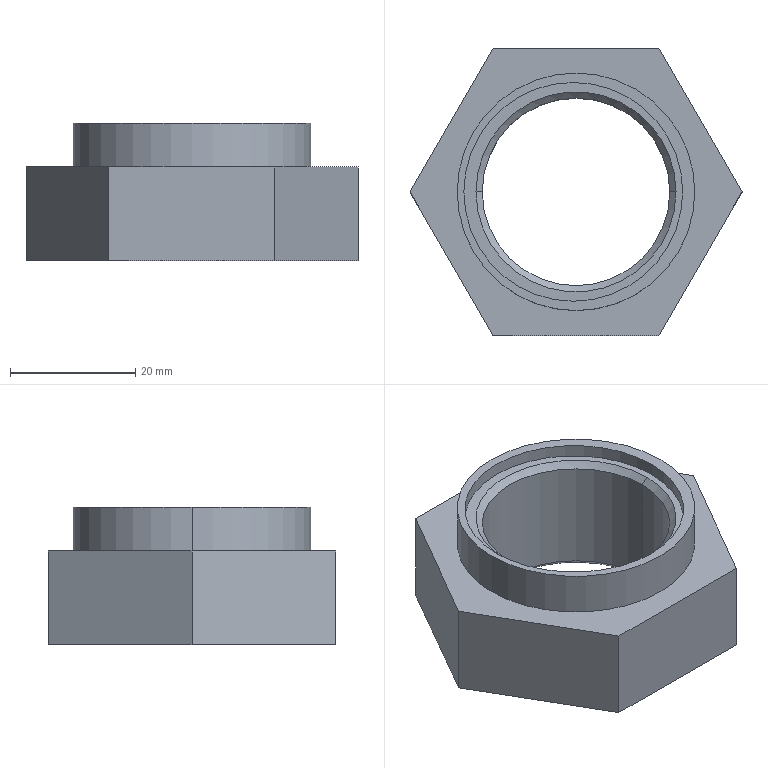Part | SolidWorks | features ICE 3, Chamfer 1, Extrusion 1 | 1 solid | 20 faces | box 53.116 x 46 x 22 mm | volume 19269 mm3 | plane 10 | cylinder 6 | cone 4 | commonest cylinder face diameters 30 x2 35 x2 38 x2
STEP:
#1=CARTESIAN_POINT('',(-15.,0.,-3.));
#2=VERTEX_POINT('',#1);
#3=CARTESIAN_POINT('',(15.,0.,-3.));
#4=VERTEX_POINT('',#3);
#5=CARTESIAN_POINT('',(0.,0.,-3.));
#6=DIRECTION('',(0.,0.,1.));
#7=DIRECTION('',(1.,0.,0.));
#8=AXIS2_PLACEMENT_3D('',#5,#6,#7);
#9=CIRCLE('',#8,15.);
#10=EDGE_CURVE('',#2,#4,#9,.T.);
#11=ORIENTED_EDGE('',*,*,#10,.F.);
#12=CARTESIAN_POINT('',(-16.,0.,-2.));
#13=VERTEX_POINT('',#12);
#14=CARTESIAN_POINT('',(-15.,0.,-3.));
#15=DIRECTION('',(-0.7071,0.,0.7071));
#16=VECTOR('',#15,1000.);
#17=LINE('',#14,#16);
#18=EDGE_CURVE('',#2,#13,#17,.T.);
#19=ORIENTED_EDGE('',*,*,#18,.T.);
#20=CARTESIAN_POINT('',(16.,0.,-2.));
#21=VERTEX_POINT('',#20);
#22=CARTESIAN_POINT('',(0.,0.,-2.));
#23=DIRECTION('',(0.,0.,-1.));
#24=DIRECTION('',(1.,0.,0.));
#25=AXIS2_PLACEMENT_3D('',#22,#23,#24);
#26=CIRCLE('',#25,16.);
#27=EDGE_CURVE('',#21,#13,#26,.T.);
#28=ORIENTED_EDGE('',*,*,#27,.F.);
#29=CARTESIAN_POINT('',(15.,0.,-3.));
#30=DIRECTION('',(0.7071,0.,0.7071));
#31=VECTOR('',#30,1000.);
#32=LINE('',#29,#31);
#33=EDGE_CURVE('',#4,#21,#32,.T.);
#34=ORIENTED_EDGE('',*,*,#33,.F.);
#35=EDGE_LOOP('',(#11,#19,#28,#34));
#36=FACE_OUTER_BOUND('',#35,.T.);
#37=CARTESIAN_POINT('',(0.,0.,-3.));
#38=DIRECTION('',(0.,0.,1.));
#39=DIRECTION('',(1.,0.,0.));
#40=AXIS2_PLACEMENT_3D('',#37,#38,#39);
#41=CONICAL_SURFACE('',#40,15.,0.7854);
#42=ADVANCED_FACE('',(#36),#41,.F.);
#43=CARTESIAN_POINT('',(15.,0.,-21.));
#44=VERTEX_POINT('',#43);
#45=CARTESIAN_POINT('',(-15.,0.,-21.));
#46=VERTEX_POINT('',#45);
#47=CARTESIAN_POINT('',(0.,0.,-21.));
#48=DIRECTION('',(0.,0.,-1.));
#49=DIRECTION('',(-1.,0.,0.));
#50=AXIS2_PLACEMENT_3D('',#47,#48,#49);
#51=CIRCLE('',#50,15.);
#52=EDGE_CURVE('',#44,#46,#51,.T.);
#53=ORIENTED_EDGE('',*,*,#52,.F.);
#54=CARTESIAN_POINT('',(16.,0.,-22.));
#55=VERTEX_POINT('',#54);
#56=CARTESIAN_POINT('',(16.,0.,-22.));
#57=DIRECTION('',(0.7071,0.,-0.7071));
#58=VECTOR('',#57,1000.);
#59=LINE('',#56,#58);
#60=EDGE_CURVE('',#44,#55,#59,.T.);
#61=ORIENTED_EDGE('',*,*,#60,.T.);
#62=CARTESIAN_POINT('',(-16.,0.,-22.));
#63=VERTEX_POINT('',#62);
#64=CARTESIAN_POINT('',(0.,0.,-22.));
#65=DIRECTION('',(0.,0.,1.));
#66=DIRECTION('',(-1.,0.,0.));
#67=AXIS2_PLACEMENT_3D('',#64,#65,#66);
#68=CIRCLE('',#67,16.);
#69=EDGE_CURVE('',#63,#55,#68,.T.);
#70=ORIENTED_EDGE('',*,*,#69,.F.);
#71=CARTESIAN_POINT('',(-16.,0.,-22.));
#72=DIRECTION('',(-0.7071,0.,-0.7071));
#73=VECTOR('',#72,1000.);
#74=LINE('',#71,#73);
#75=EDGE_CURVE('',#46,#63,#74,.T.);
#76=ORIENTED_EDGE('',*,*,#75,.F.);
#77=EDGE_LOOP('',(#53,#61,#70,#76));
#78=FACE_OUTER_BOUND('',#77,.T.);
#79=CARTESIAN_POINT('',(0.,0.,-22.));
#80=DIRECTION('',(0.,0.,-1.));
#81=DIRECTION('',(-1.,0.,0.));
#82=AXIS2_PLACEMENT_3D('',#79,#80,#81);
#83=CONICAL_SURFACE('',#82,16.,0.7854);
#84=ADVANCED_FACE('',(#78),#83,.F.);
#85=ORIENTED_EDGE('',*,*,#52,.T.);
#86=CARTESIAN_POINT('',(-15.,0.,-22.));
#87=DIRECTION('',(0.,0.,1.));
#88=VECTOR('',#87,1000.);
#89=LINE('',#86,#88);
#90=EDGE_CURVE('',#46,#2,#89,.T.);
#91=ORIENTED_EDGE('',*,*,#90,.T.);
#92=ORIENTED_EDGE('',*,*,#10,.T.);
#93=CARTESIAN_POINT('',(15.,0.,-22.));
#94=DIRECTION('',(0.,0.,1.));
#95=VECTOR('',#94,1000.);
#96=LINE('',#93,#95);
#97=EDGE_CURVE('',#44,#4,#96,.T.);
#98=ORIENTED_EDGE('',*,*,#97,.F.);
#99=EDGE_LOOP('',(#85,#91,#92,#98));
#100=FACE_OUTER_BOUND('',#99,.T.);
#101=CARTESIAN_POINT('',(0.,0.,-22.));
#102=DIRECTION('',(0.,0.,1.));
#103=DIRECTION('',(1.,0.,0.));
#104=AXIS2_PLACEMENT_3D('',#101,#102,#103);
#105=CYLINDRICAL_SURFACE('',#104,15.);
#106=ADVANCED_FACE('',(#100),#105,.F.);
#107=CARTESIAN_POINT('',(-17.937,0.,-2.));
#108=VERTEX_POINT('',#107);
#109=CARTESIAN_POINT('',(17.063,0.,-2.));
#110=VERTEX_POINT('',#109);
#111=CARTESIAN_POINT('',(-0.4374,0.,-2.));
#112=DIRECTION('',(0.,0.,1.));
#113=DIRECTION('',(1.,0.,0.));
#114=AXIS2_PLACEMENT_3D('',#111,#112,#113);
#115=CIRCLE('',#114,17.5);
#116=EDGE_CURVE('',#108,#110,#115,.T.);
#117=ORIENTED_EDGE('',*,*,#116,.F.);
#118=CARTESIAN_POINT('',(-17.937,0.,0.));
#119=VERTEX_POINT('',#118);
#120=CARTESIAN_POINT('',(-17.937,0.,-2.));
#121=DIRECTION('',(0.,0.,1.));
#122=VECTOR('',#121,1000.);
#123=LINE('',#120,#122);
#124=EDGE_CURVE('',#108,#119,#123,.T.);
#125=ORIENTED_EDGE('',*,*,#124,.T.);
#126=CARTESIAN_POINT('',(17.063,0.,0.));
#127=VERTEX_POINT('',#126);
#128=CARTESIAN_POINT('',(-0.4374,0.,0.));
#129=DIRECTION('',(0.,0.,1.));
#130=DIRECTION('',(1.,0.,0.));
#131=AXIS2_PLACEMENT_3D('',#128,#129,#130);
#132=CIRCLE('',#131,17.5);
#133=EDGE_CURVE('',#119,#127,#132,.T.);
#134=ORIENTED_EDGE('',*,*,#133,.T.);
#135=CARTESIAN_POINT('',(17.063,0.,-2.));
#136=DIRECTION('',(0.,0.,1.));
#137=VECTOR('',#136,1000.);
#138=LINE('',#135,#137);
#139=EDGE_CURVE('',#110,#127,#138,.T.);
#140=ORIENTED_EDGE('',*,*,#139,.F.);
#141=EDGE_LOOP('',(#117,#125,#134,#140));
#142=FACE_OUTER_BOUND('',#141,.T.);
#143=CARTESIAN_POINT('',(-0.4374,0.,-2.));
#144=DIRECTION('',(0.,0.,1.));
#145=DIRECTION('',(1.,0.,0.));
#146=AXIS2_PLACEMENT_3D('',#143,#144,#145);
#147=CYLINDRICAL_SURFACE('',#146,17.5);
#148=ADVANCED_FACE('',(#142),#147,.F.);
#149=CARTESIAN_POINT('',(19.,0.,-7.));
#150=VERTEX_POINT('',#149);
#151=CARTESIAN_POINT('',(-19.,0.,-7.));
#152=VERTEX_POINT('',#151);
#153=CARTESIAN_POINT('',(0.,0.,-7.));
#154=DIRECTION('',(0.,0.,1.));
#155=DIRECTION('',(-1.,0.,0.));
#156=AXIS2_PLACEMENT_3D('',#153,#154,#155);
#157=CIRCLE('',#156,19.);
#158=EDGE_CURVE('',#150,#152,#157,.T.);
#159=ORIENTED_EDGE('',*,*,#158,.T.);
#160=CARTESIAN_POINT('',(-19.,0.,0.));
#161=VERTEX_POINT('',#160);
#162=CARTESIAN_POINT('',(-19.,0.,-7.));
#163=DIRECTION('',(0.,0.,1.));
#164=VECTOR('',#163,1000.);
#165=LINE('',#162,#164);
#166=EDGE_CURVE('',#152,#161,#165,.T.);
#167=ORIENTED_EDGE('',*,*,#166,.T.);
#168=CARTESIAN_POINT('',(19.,0.,0.));
#169=VERTEX_POINT('',#168);
#170=CARTESIAN_POINT('',(0.,0.,0.));
#171=DIRECTION('',(0.,0.,1.));
#172=DIRECTION('',(1.,0.,0.));
#173=AXIS2_PLACEMENT_3D('',#170,#171,#172);
#174=CIRCLE('',#173,19.);
#175=EDGE_CURVE('',#169,#161,#174,.T.);
#176=ORIENTED_EDGE('',*,*,#175,.F.);
#177=CARTESIAN_POINT('',(19.,0.,-7.));
#178=DIRECTION('',(0.,0.,1.));
#179=VECTOR('',#178,1000.);
#180=LINE('',#177,#179);
#181=EDGE_CURVE('',#150,#169,#180,.T.);
#182=ORIENTED_EDGE('',*,*,#181,.F.);
#183=EDGE_LOOP('',(#159,#167,#176,#182));
#184=FACE_OUTER_BOUND('',#183,.T.);
#185=CARTESIAN_POINT('',(0.,0.,-7.));
#186=DIRECTION('',(0.,0.,1.));
#187=DIRECTION('',(1.,0.,0.));
#188=AXIS2_PLACEMENT_3D('',#185,#186,#187);
#189=CYLINDRICAL_SURFACE('',#188,19.);
#190=ADVANCED_FACE('',(#184),#189,.T.);
#191=ORIENTED_EDGE('',*,*,#166,.F.);
#192=CARTESIAN_POINT('',(0.,0.,-7.));
#193=DIRECTION('',(0.,0.,1.));
#194=DIRECTION('',(-1.,0.,0.));
#195=AXIS2_PLACEMENT_3D('',#192,#193,#194);
#196=CIRCLE('',#195,19.);
#197=EDGE_CURVE('',#152,#150,#196,.T.);
#198=ORIENTED_EDGE('',*,*,#197,.T.);
#199=ORIENTED_EDGE('',*,*,#181,.T.);
#200=CARTESIAN_POINT('',(0.,0.,0.));
#201=DIRECTION('',(0.,0.,1.));
#202=DIRECTION('',(1.,0.,0.));
#203=AXIS2_PLACEMENT_3D('',#200,#201,#202);
#204=CIRCLE('',#203,19.);
#205=EDGE_CURVE('',#161,#169,#204,.T.);
#206=ORIENTED_EDGE('',*,*,#205,.F.);
#207=EDGE_LOOP('',(#191,#198,#199,#206));
#208=FACE_OUTER_BOUND('',#207,.T.);
#209=CARTESIAN_POINT('',(0.,0.,-7.));
#210=DIRECTION('',(0.,0.,1.));
#211=DIRECTION('',(1.,0.,0.));
#212=AXIS2_PLACEMENT_3D('',#209,#210,#211);
#213=CYLINDRICAL_SURFACE('',#212,19.);
#214=ADVANCED_FACE('',(#208),#213,.T.);
#215=CARTESIAN_POINT('',(-0.4374,0.,0.));
#216=DIRECTION('',(0.,0.,1.));
#217=DIRECTION('',(1.,0.,0.));
#218=AXIS2_PLACEMENT_3D('',#215,#216,#217);
#219=CIRCLE('',#218,17.5);
#220=EDGE_CURVE('',#127,#119,#219,.T.);
#221=ORIENTED_EDGE('',*,*,#220,.F.);
#222=ORIENTED_EDGE('',*,*,#133,.F.);
#223=EDGE_LOOP('',(#221,#222));
#224=FACE_BOUND('',#223,.T.);
#225=ORIENTED_EDGE('',*,*,#175,.T.);
#226=ORIENTED_EDGE('',*,*,#205,.T.);
#227=EDGE_LOOP('',(#225,#226));
#228=FACE_OUTER_BOUND('',#227,.T.);
#229=CARTESIAN_POINT('',(0.,0.,0.));
#230=DIRECTION('',(0.,0.,1.));
#231=DIRECTION('',(1.,0.,0.));
#232=AXIS2_PLACEMENT_3D('',#229,#230,#231);
#233=PLANE('',#232);
#234=ADVANCED_FACE('',(#224,#228),#233,.T.);
#235=CARTESIAN_POINT('',(13.279,-23.,-7.));
#236=VERTEX_POINT('',#235);
#237=CARTESIAN_POINT('',(-13.279,-23.,-7.));
#238=VERTEX_POINT('',#237);
#239=CARTESIAN_POINT('',(13.279,-23.,-7.));
#240=DIRECTION('',(-1.,0.,0.));
#241=VECTOR('',#240,1000.);
#242=LINE('',#239,#241);
#243=EDGE_CURVE('',#236,#238,#242,.T.);
#244=ORIENTED_EDGE('',*,*,#243,.T.);
#245=CARTESIAN_POINT('',(-13.279,-23.,-22.));
#246=VERTEX_POINT('',#245);
#247=CARTESIAN_POINT('',(-13.279,-23.,-22.));
#248=DIRECTION('',(0.,0.,1.));
#249=VECTOR('',#248,1000.);
#250=LINE('',#247,#249);
#251=EDGE_CURVE('',#246,#238,#250,.T.);
#252=ORIENTED_EDGE('',*,*,#251,.F.);
#253=CARTESIAN_POINT('',(13.279,-23.,-22.));
#254=VERTEX_POINT('',#253);
#255=CARTESIAN_POINT('',(13.279,-23.,-22.));
#256=DIRECTION('',(-1.,0.,0.));
#257=VECTOR('',#256,1000.);
#258=LINE('',#255,#257);
#259=EDGE_CURVE('',#254,#246,#258,.T.);
#260=ORIENTED_EDGE('',*,*,#259,.F.);
#261=CARTESIAN_POINT('',(13.279,-23.,-22.));
#262=DIRECTION('',(0.,0.,1.));
#263=VECTOR('',#262,1000.);
#264=LINE('',#261,#263);
#265=EDGE_CURVE('',#254,#236,#264,.T.);
#266=ORIENTED_EDGE('',*,*,#265,.T.);
#267=EDGE_LOOP('',(#244,#252,#260,#266));
#268=FACE_OUTER_BOUND('',#267,.T.);
#269=CARTESIAN_POINT('',(13.279,-23.,-22.));
#270=DIRECTION('',(0.,1.,0.));
#271=DIRECTION('',(0.,0.,1.));
#272=AXIS2_PLACEMENT_3D('',#269,#270,#271);
#273=PLANE('',#272);
#274=ADVANCED_FACE('',(#268),#273,.F.);
#275=CARTESIAN_POINT('',(-26.558,0.,-7.));
#276=VERTEX_POINT('',#275);
#277=CARTESIAN_POINT('',(-13.279,-23.,-7.));
#278=DIRECTION('',(-0.5,0.866,0.));
#279=VECTOR('',#278,1000.);
#280=LINE('',#277,#279);
#281=EDGE_CURVE('',#238,#276,#280,.T.);
#282=ORIENTED_EDGE('',*,*,#281,.T.);
#283=CARTESIAN_POINT('',(-26.558,0.,-22.));
#284=VERTEX_POINT('',#283);
#285=CARTESIAN_POINT('',(-26.558,0.,-22.));
#286=DIRECTION('',(0.,0.,1.));
#287=VECTOR('',#286,1000.);
#288=LINE('',#285,#287);
#289=EDGE_CURVE('',#284,#276,#288,.T.);
#290=ORIENTED_EDGE('',*,*,#289,.F.);
#291=CARTESIAN_POINT('',(-13.279,-23.,-22.));
#292=DIRECTION('',(-0.5,0.866,0.));
#293=VECTOR('',#292,1000.);
#294=LINE('',#291,#293);
#295=EDGE_CURVE('',#246,#284,#294,.T.);
#296=ORIENTED_EDGE('',*,*,#295,.F.);
#297=ORIENTED_EDGE('',*,*,#251,.T.);
#298=EDGE_LOOP('',(#282,#290,#296,#297));
#299=FACE_OUTER_BOUND('',#298,.T.);
#300=CARTESIAN_POINT('',(-13.279,-23.,-22.));
#301=DIRECTION('',(0.866,0.5,0.));
#302=DIRECTION('',(-0.5,0.866,0.));
#303=AXIS2_PLACEMENT_3D('',#300,#301,#302);
#304=PLANE('',#303);
#305=ADVANCED_FACE('',(#299),#304,.F.);
#306=CARTESIAN_POINT('',(-13.279,23.,-7.));
#307=VERTEX_POINT('',#306);
#308=CARTESIAN_POINT('',(-26.558,0.,-7.));
#309=DIRECTION('',(0.5,0.866,0.));
#310=VECTOR('',#309,1000.);
#311=LINE('',#308,#310);
#312=EDGE_CURVE('',#276,#307,#311,.T.);
#313=ORIENTED_EDGE('',*,*,#312,.T.);
#314=CARTESIAN_POINT('',(-13.279,23.,-22.));
#315=VERTEX_POINT('',#314);
#316=CARTESIAN_POINT('',(-13.279,23.,-22.));
#317=DIRECTION('',(0.,0.,1.));
#318=VECTOR('',#317,1000.);
#319=LINE('',#316,#318);
#320=EDGE_CURVE('',#315,#307,#319,.T.);
#321=ORIENTED_EDGE('',*,*,#320,.F.);
#322=CARTESIAN_POINT('',(-26.558,0.,-22.));
#323=DIRECTION('',(0.5,0.866,0.));
#324=VECTOR('',#323,1000.);
#325=LINE('',#322,#324);
#326=EDGE_CURVE('',#284,#315,#325,.T.);
#327=ORIENTED_EDGE('',*,*,#326,.F.);
#328=ORIENTED_EDGE('',*,*,#289,.T.);
#329=EDGE_LOOP('',(#313,#321,#327,#328));
#330=FACE_OUTER_BOUND('',#329,.T.);
#331=CARTESIAN_POINT('',(-26.558,0.,-22.));
#332=DIRECTION('',(0.866,-0.5,0.));
#333=DIRECTION('',(0.5,0.866,0.));
#334=AXIS2_PLACEMENT_3D('',#331,#332,#333);
#335=PLANE('',#334);
#336=ADVANCED_FACE('',(#330),#335,.F.);
#337=CARTESIAN_POINT('',(13.279,23.,-7.));
#338=VERTEX_POINT('',#337);
#339=CARTESIAN_POINT('',(-13.279,23.,-7.));
#340=DIRECTION('',(1.,0.,0.));
#341=VECTOR('',#340,1000.);
#342=LINE('',#339,#341);
#343=EDGE_CURVE('',#307,#338,#342,.T.);
#344=ORIENTED_EDGE('',*,*,#343,.T.);
#345=CARTESIAN_POINT('',(13.279,23.,-22.));
#346=VERTEX_POINT('',#345);
#347=CARTESIAN_POINT('',(13.279,23.,-22.));
#348=DIRECTION('',(0.,0.,1.));
#349=VECTOR('',#348,1000.);
#350=LINE('',#347,#349);
#351=EDGE_CURVE('',#346,#338,#350,.T.);
#352=ORIENTED_EDGE('',*,*,#351,.F.);
#353=CARTESIAN_POINT('',(-13.279,23.,-22.));
#354=DIRECTION('',(1.,0.,0.));
#355=VECTOR('',#354,1000.);
#356=LINE('',#353,#355);
#357=EDGE_CURVE('',#315,#346,#356,.T.);
#358=ORIENTED_EDGE('',*,*,#357,.F.);
#359=ORIENTED_EDGE('',*,*,#320,.T.);
#360=EDGE_LOOP('',(#344,#352,#358,#359));
#361=FACE_OUTER_BOUND('',#360,.T.);
#362=CARTESIAN_POINT('',(-13.279,23.,-22.));
#363=DIRECTION('',(0.,-1.,0.));
#364=DIRECTION('',(0.,0.,-1.));
#365=AXIS2_PLACEMENT_3D('',#362,#363,#364);
#366=PLANE('',#365);
#367=ADVANCED_FACE('',(#361),#366,.F.);
#368=CARTESIAN_POINT('',(26.558,0.,-7.));
#369=VERTEX_POINT('',#368);
#370=CARTESIAN_POINT('',(13.279,23.,-7.));
#371=DIRECTION('',(0.5,-0.866,0.));
#372=VECTOR('',#371,1000.);
#373=LINE('',#370,#372);
#374=EDGE_CURVE('',#338,#369,#373,.T.);
#375=ORIENTED_EDGE('',*,*,#374,.T.);
#376=CARTESIAN_POINT('',(26.558,0.,-22.));
#377=VERTEX_POINT('',#376);
#378=CARTESIAN_POINT('',(26.558,0.,-22.));
#379=DIRECTION('',(0.,0.,1.));
#380=VECTOR('',#379,1000.);
#381=LINE('',#378,#380);
#382=EDGE_CURVE('',#377,#369,#381,.T.);
#383=ORIENTED_EDGE('',*,*,#382,.F.);
#384=CARTESIAN_POINT('',(13.279,23.,-22.));
#385=DIRECTION('',(0.5,-0.866,0.));
#386=VECTOR('',#385,1000.);
#387=LINE('',#384,#386);
#388=EDGE_CURVE('',#346,#377,#387,.T.);
#389=ORIENTED_EDGE('',*,*,#388,.F.);
#390=ORIENTED_EDGE('',*,*,#351,.T.);
#391=EDGE_LOOP('',(#375,#383,#389,#390));
#392=FACE_OUTER_BOUND('',#391,.T.);
#393=CARTESIAN_POINT('',(13.279,23.,-22.));
#394=DIRECTION('',(-0.866,-0.5,0.));
#395=DIRECTION('',(0.5,-0.866,0.));
#396=AXIS2_PLACEMENT_3D('',#393,#394,#395);
#397=PLANE('',#396);
#398=ADVANCED_FACE('',(#392),#397,.F.);
#399=CARTESIAN_POINT('',(26.558,0.,-7.));
#400=DIRECTION('',(-0.5,-0.866,0.));
#401=VECTOR('',#400,1000.);
#402=LINE('',#399,#401);
#403=EDGE_CURVE('',#369,#236,#402,.T.);
#404=ORIENTED_EDGE('',*,*,#403,.T.);
#405=ORIENTED_EDGE('',*,*,#265,.F.);
#406=CARTESIAN_POINT('',(26.558,0.,-22.));
#407=DIRECTION('',(-0.5,-0.866,0.));
#408=VECTOR('',#407,1000.);
#409=LINE('',#406,#408);
#410=EDGE_CURVE('',#377,#254,#409,.T.);
#411=ORIENTED_EDGE('',*,*,#410,.F.);
#412=ORIENTED_EDGE('',*,*,#382,.T.);
#413=EDGE_LOOP('',(#404,#405,#411,#412));
#414=FACE_OUTER_BOUND('',#413,.T.);
#415=CARTESIAN_POINT('',(26.558,0.,-22.));
#416=DIRECTION('',(-0.866,0.5,0.));
#417=DIRECTION('',(-0.5,-0.866,0.));
#418=AXIS2_PLACEMENT_3D('',#415,#416,#417);
#419=PLANE('',#418);
#420=ADVANCED_FACE('',(#414),#419,.F.);
#421=ORIENTED_EDGE('',*,*,#69,.T.);
#422=CARTESIAN_POINT('',(0.,0.,-22.));
#423=DIRECTION('',(0.,0.,1.));
#424=DIRECTION('',(-1.,0.,0.));
#425=AXIS2_PLACEMENT_3D('',#422,#423,#424);
#426=CIRCLE('',#425,16.);
#427=EDGE_CURVE('',#55,#63,#426,.T.);
#428=ORIENTED_EDGE('',*,*,#427,.T.);
#429=EDGE_LOOP('',(#421,#428));
#430=FACE_BOUND('',#429,.T.);
#431=ORIENTED_EDGE('',*,*,#259,.T.);
#432=ORIENTED_EDGE('',*,*,#295,.T.);
#433=ORIENTED_EDGE('',*,*,#326,.T.);
#434=ORIENTED_EDGE('',*,*,#357,.T.);
#435=ORIENTED_EDGE('',*,*,#388,.T.);
#436=ORIENTED_EDGE('',*,*,#410,.T.);
#437=EDGE_LOOP('',(#431,#432,#433,#434,#435,#436));
#438=FACE_OUTER_BOUND('',#437,.T.);
#439=CARTESIAN_POINT('',(0.,0.,-22.));
#440=DIRECTION('',(0.,0.,-1.));
#441=DIRECTION('',(-1.,0.,0.));
#442=AXIS2_PLACEMENT_3D('',#439,#440,#441);
#443=PLANE('',#442);
#444=ADVANCED_FACE('',(#430,#438),#443,.T.);
#445=ORIENTED_EDGE('',*,*,#158,.F.);
#446=ORIENTED_EDGE('',*,*,#197,.F.);
#447=EDGE_LOOP('',(#445,#446));
#448=FACE_BOUND('',#447,.T.);
#449=ORIENTED_EDGE('',*,*,#243,.F.);
#450=ORIENTED_EDGE('',*,*,#403,.F.);
#451=ORIENTED_EDGE('',*,*,#374,.F.);
#452=ORIENTED_EDGE('',*,*,#343,.F.);
#453=ORIENTED_EDGE('',*,*,#312,.F.);
#454=ORIENTED_EDGE('',*,*,#281,.F.);
#455=EDGE_LOOP('',(#449,#450,#451,#452,#453,#454));
#456=FACE_OUTER_BOUND('',#455,.T.);
#457=CARTESIAN_POINT('',(0.,0.,-7.));
#458=DIRECTION('',(0.,0.,-1.));
#459=DIRECTION('',(-1.,0.,0.));
#460=AXIS2_PLACEMENT_3D('',#457,#458,#459);
#461=PLANE('',#460);
#462=ADVANCED_FACE('',(#448,#456),#461,.F.);
#463=ORIENTED_EDGE('',*,*,#124,.F.);
#464=CARTESIAN_POINT('',(-0.4374,0.,-2.));
#465=DIRECTION('',(0.,0.,1.));
#466=DIRECTION('',(1.,0.,0.));
#467=AXIS2_PLACEMENT_3D('',#464,#465,#466);
#468=CIRCLE('',#467,17.5);
#469=EDGE_CURVE('',#110,#108,#468,.T.);
#470=ORIENTED_EDGE('',*,*,#469,.F.);
#471=ORIENTED_EDGE('',*,*,#139,.T.);
#472=ORIENTED_EDGE('',*,*,#220,.T.);
#473=EDGE_LOOP('',(#463,#470,#471,#472));
#474=FACE_OUTER_BOUND('',#473,.T.);
#475=CARTESIAN_POINT('',(-0.4374,0.,-2.));
#476=DIRECTION('',(0.,0.,1.));
#477=DIRECTION('',(1.,0.,0.));
#478=AXIS2_PLACEMENT_3D('',#475,#476,#477);
#479=CYLINDRICAL_SURFACE('',#478,17.5);
#480=ADVANCED_FACE('',(#474),#479,.F.);
#481=ORIENTED_EDGE('',*,*,#27,.T.);
#482=CARTESIAN_POINT('',(0.,0.,-2.));
#483=DIRECTION('',(0.,0.,-1.));
#484=DIRECTION('',(1.,0.,0.));
#485=AXIS2_PLACEMENT_3D('',#482,#483,#484);
#486=CIRCLE('',#485,16.);
#487=EDGE_CURVE('',#13,#21,#486,.T.);
#488=ORIENTED_EDGE('',*,*,#487,.T.);
#489=EDGE_LOOP('',(#481,#488));
#490=FACE_BOUND('',#489,.T.);
#491=ORIENTED_EDGE('',*,*,#469,.T.);
#492=ORIENTED_EDGE('',*,*,#116,.T.);
#493=EDGE_LOOP('',(#491,#492));
#494=FACE_OUTER_BOUND('',#493,.T.);
#495=CARTESIAN_POINT('',(-0.4374,0.,-2.));
#496=DIRECTION('',(0.,0.,1.));
#497=DIRECTION('',(1.,0.,0.));
#498=AXIS2_PLACEMENT_3D('',#495,#496,#497);
#499=PLANE('',#498);
#500=ADVANCED_FACE('',(#490,#494),#499,.T.);
#501=ORIENTED_EDGE('',*,*,#90,.F.);
#502=CARTESIAN_POINT('',(0.,0.,-21.));
#503=DIRECTION('',(0.,0.,-1.));
#504=DIRECTION('',(-1.,0.,0.));
#505=AXIS2_PLACEMENT_3D('',#502,#503,#504);
#506=CIRCLE('',#505,15.);
#507=EDGE_CURVE('',#46,#44,#506,.T.);
#508=ORIENTED_EDGE('',*,*,#507,.T.);
#509=ORIENTED_EDGE('',*,*,#97,.T.);
#510=CARTESIAN_POINT('',(0.,0.,-3.));
#511=DIRECTION('',(0.,0.,1.));
#512=DIRECTION('',(1.,0.,0.));
#513=AXIS2_PLACEMENT_3D('',#510,#511,#512);
#514=CIRCLE('',#513,15.);
#515=EDGE_CURVE('',#4,#2,#514,.T.);
#516=ORIENTED_EDGE('',*,*,#515,.T.);
#517=EDGE_LOOP('',(#501,#508,#509,#516));
#518=FACE_OUTER_BOUND('',#517,.T.);
#519=CARTESIAN_POINT('',(0.,0.,-22.));
#520=DIRECTION('',(0.,0.,1.));
#521=DIRECTION('',(1.,0.,0.));
#522=AXIS2_PLACEMENT_3D('',#519,#520,#521);
#523=CYLINDRICAL_SURFACE('',#522,15.);
#524=ADVANCED_FACE('',(#518),#523,.F.);
#525=ORIENTED_EDGE('',*,*,#60,.F.);
#526=ORIENTED_EDGE('',*,*,#507,.F.);
#527=ORIENTED_EDGE('',*,*,#75,.T.);
#528=ORIENTED_EDGE('',*,*,#427,.F.);
#529=EDGE_LOOP('',(#525,#526,#527,#528));
#530=FACE_OUTER_BOUND('',#529,.T.);
#531=CARTESIAN_POINT('',(0.,0.,-22.));
#532=DIRECTION('',(0.,0.,-1.));
#533=DIRECTION('',(-1.,0.,0.));
#534=AXIS2_PLACEMENT_3D('',#531,#532,#533);
#535=CONICAL_SURFACE('',#534,16.,0.7854);
#536=ADVANCED_FACE('',(#530),#535,.F.);
#537=ORIENTED_EDGE('',*,*,#18,.F.);
#538=ORIENTED_EDGE('',*,*,#515,.F.);
#539=ORIENTED_EDGE('',*,*,#33,.T.);
#540=ORIENTED_EDGE('',*,*,#487,.F.);
#541=EDGE_LOOP('',(#537,#538,#539,#540));
#542=FACE_OUTER_BOUND('',#541,.T.);
#543=CARTESIAN_POINT('',(0.,0.,-3.));
#544=DIRECTION('',(0.,0.,1.));
#545=DIRECTION('',(1.,0.,0.));
#546=AXIS2_PLACEMENT_3D('',#543,#544,#545);
#547=CONICAL_SURFACE('',#546,15.,0.7854);
#548=ADVANCED_FACE('',(#542),#547,.F.);
#549=CLOSED_SHELL('',(#42,#84,#106,#148,#190,#214,#234,#274,#305,#336,#367,#398,#420,#444,#462,#480,#500,#524,#536,#548));
#550=MANIFOLD_SOLID_BREP('',#549);
#551=CARTESIAN_POINT('',(0.,0.,0.));
#552=DIRECTION('',(0.,0.,1.));
#553=DIRECTION('',(1.,0.,0.));
#554=AXIS2_PLACEMENT_3D('',#551,#552,#553);
#555=(LENGTH_UNIT()NAMED_UNIT(*)SI_UNIT(.MILLI.,.METRE.));
#556=UNCERTAINTY_MEASURE_WITH_UNIT(LENGTH_MEASURE(0.00001),#555,'','');
#557=(NAMED_UNIT(*)PLANE_ANGLE_UNIT()SI_UNIT($,.RADIAN.));
#558=(NAMED_UNIT(*)SI_UNIT($,.STERADIAN.)SOLID_ANGLE_UNIT());
#559=(GEOMETRIC_REPRESENTATION_CONTEXT(3)GLOBAL_UNCERTAINTY_ASSIGNED_CONTEXT((#556))GLOBAL_UNIT_ASSIGNED_CONTEXT((#555,#557,#558))REPRESENTATION_CONTEXT('',''));
#560=ADVANCED_BREP_SHAPE_REPRESENTATION('',(#550,#554),#559);